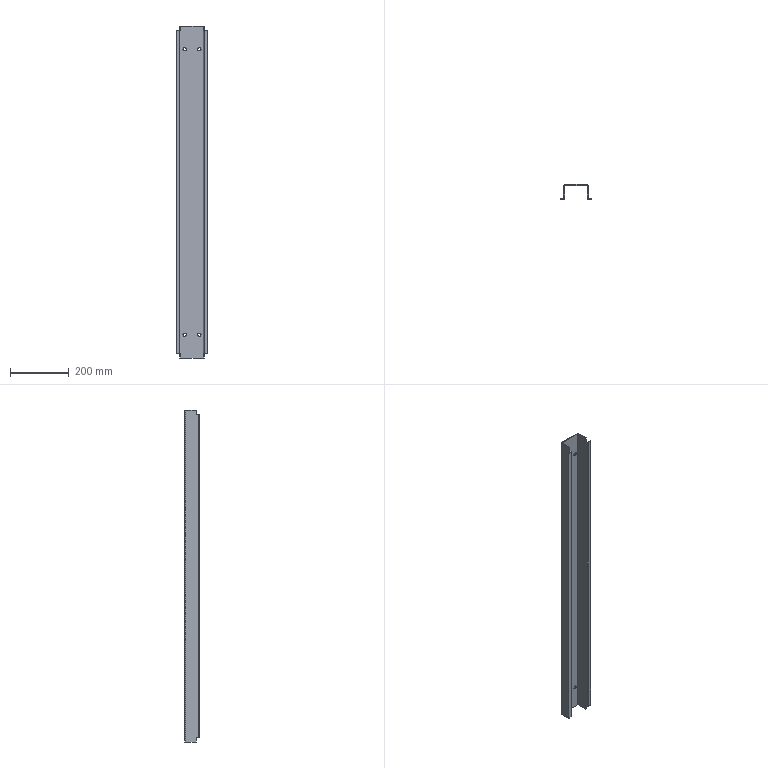Part | SolidWorks | features ICE 3, Chamfer 1, Cut 1, FlatPattern 1, SMBaseFlange 1, SheetMetal 1 | 1 solid | 54 faces | box 106 x 50 x 1127 mm | volume 661257 mm3 | plane 38 | cylinder 16 | commonest cylinder face diameters 11.5 x8 0.4 x4 6.4 x4
STEP:
#1=CARTESIAN_POINT('',(-25.,-3.,478.75));
#2=VERTEX_POINT('',#1);
#3=CARTESIAN_POINT('',(-25.,-3.,490.25));
#4=VERTEX_POINT('',#3);
#5=CARTESIAN_POINT('',(-25.,-3.,484.5));
#6=DIRECTION('',(0.,1.,0.));
#7=DIRECTION('',(-1.,0.,0.));
#8=AXIS2_PLACEMENT_3D('',#5,#6,#7);
#9=CIRCLE('',#8,5.75);
#10=EDGE_CURVE('',#2,#4,#9,.T.);
#11=ORIENTED_EDGE('',*,*,#10,.F.);
#12=CARTESIAN_POINT('',(-25.,0.,478.75));
#13=VERTEX_POINT('',#12);
#14=CARTESIAN_POINT('',(-25.,-10.,478.75));
#15=DIRECTION('',(0.,1.,0.));
#16=VECTOR('',#15,1000.);
#17=LINE('',#14,#16);
#18=EDGE_CURVE('',#2,#13,#17,.T.);
#19=ORIENTED_EDGE('',*,*,#18,.T.);
#20=CARTESIAN_POINT('',(-25.,0.,490.25));
#21=VERTEX_POINT('',#20);
#22=CARTESIAN_POINT('',(-25.,0.,484.5));
#23=DIRECTION('',(0.,1.,0.));
#24=DIRECTION('',(0.,0.,1.));
#25=AXIS2_PLACEMENT_3D('',#22,#23,#24);
#26=CIRCLE('',#25,5.75);
#27=EDGE_CURVE('',#13,#21,#26,.T.);
#28=ORIENTED_EDGE('',*,*,#27,.T.);
#29=CARTESIAN_POINT('',(-25.,-10.,490.25));
#30=DIRECTION('',(0.,1.,0.));
#31=VECTOR('',#30,1000.);
#32=LINE('',#29,#31);
#33=EDGE_CURVE('',#4,#21,#32,.T.);
#34=ORIENTED_EDGE('',*,*,#33,.F.);
#35=EDGE_LOOP('',(#11,#19,#28,#34));
#36=FACE_OUTER_BOUND('',#35,.T.);
#37=CARTESIAN_POINT('',(-25.,-10.,484.5));
#38=DIRECTION('',(0.,1.,0.));
#39=DIRECTION('',(0.,0.,1.));
#40=AXIS2_PLACEMENT_3D('',#37,#38,#39);
#41=CYLINDRICAL_SURFACE('',#40,5.75);
#42=ADVANCED_FACE('',(#36),#41,.F.);
#43=CARTESIAN_POINT('',(25.,-3.,-490.25));
#44=VERTEX_POINT('',#43);
#45=CARTESIAN_POINT('',(25.,-3.,-478.75));
#46=VERTEX_POINT('',#45);
#47=CARTESIAN_POINT('',(25.,-3.,-484.5));
#48=DIRECTION('',(0.,1.,0.));
#49=DIRECTION('',(-1.,0.,0.));
#50=AXIS2_PLACEMENT_3D('',#47,#48,#49);
#51=CIRCLE('',#50,5.75);
#52=EDGE_CURVE('',#44,#46,#51,.T.);
#53=ORIENTED_EDGE('',*,*,#52,.F.);
#54=CARTESIAN_POINT('',(25.,0.,-490.25));
#55=VERTEX_POINT('',#54);
#56=CARTESIAN_POINT('',(25.,-10.,-490.25));
#57=DIRECTION('',(0.,1.,0.));
#58=VECTOR('',#57,1000.);
#59=LINE('',#56,#58);
#60=EDGE_CURVE('',#44,#55,#59,.T.);
#61=ORIENTED_EDGE('',*,*,#60,.T.);
#62=CARTESIAN_POINT('',(25.,0.,-478.75));
#63=VERTEX_POINT('',#62);
#64=CARTESIAN_POINT('',(25.,0.,-484.5));
#65=DIRECTION('',(0.,1.,0.));
#66=DIRECTION('',(0.,0.,1.));
#67=AXIS2_PLACEMENT_3D('',#64,#65,#66);
#68=CIRCLE('',#67,5.75);
#69=EDGE_CURVE('',#55,#63,#68,.T.);
#70=ORIENTED_EDGE('',*,*,#69,.T.);
#71=CARTESIAN_POINT('',(25.,-10.,-478.75));
#72=DIRECTION('',(0.,1.,0.));
#73=VECTOR('',#72,1000.);
#74=LINE('',#71,#73);
#75=EDGE_CURVE('',#46,#63,#74,.T.);
#76=ORIENTED_EDGE('',*,*,#75,.F.);
#77=EDGE_LOOP('',(#53,#61,#70,#76));
#78=FACE_OUTER_BOUND('',#77,.T.);
#79=CARTESIAN_POINT('',(25.,-10.,-484.5));
#80=DIRECTION('',(0.,1.,0.));
#81=DIRECTION('',(0.,0.,1.));
#82=AXIS2_PLACEMENT_3D('',#79,#80,#81);
#83=CYLINDRICAL_SURFACE('',#82,5.75);
#84=ADVANCED_FACE('',(#78),#83,.F.);
#85=CARTESIAN_POINT('',(25.,-3.,478.75));
#86=VERTEX_POINT('',#85);
#87=CARTESIAN_POINT('',(25.,-3.,490.25));
#88=VERTEX_POINT('',#87);
#89=CARTESIAN_POINT('',(25.,-3.,484.5));
#90=DIRECTION('',(0.,1.,0.));
#91=DIRECTION('',(-1.,0.,0.));
#92=AXIS2_PLACEMENT_3D('',#89,#90,#91);
#93=CIRCLE('',#92,5.75);
#94=EDGE_CURVE('',#86,#88,#93,.T.);
#95=ORIENTED_EDGE('',*,*,#94,.F.);
#96=CARTESIAN_POINT('',(25.,0.,478.75));
#97=VERTEX_POINT('',#96);
#98=CARTESIAN_POINT('',(25.,-10.,478.75));
#99=DIRECTION('',(0.,1.,0.));
#100=VECTOR('',#99,1000.);
#101=LINE('',#98,#100);
#102=EDGE_CURVE('',#86,#97,#101,.T.);
#103=ORIENTED_EDGE('',*,*,#102,.T.);
#104=CARTESIAN_POINT('',(25.,0.,490.25));
#105=VERTEX_POINT('',#104);
#106=CARTESIAN_POINT('',(25.,0.,484.5));
#107=DIRECTION('',(0.,1.,0.));
#108=DIRECTION('',(0.,0.,-1.));
#109=AXIS2_PLACEMENT_3D('',#106,#107,#108);
#110=CIRCLE('',#109,5.75);
#111=EDGE_CURVE('',#97,#105,#110,.T.);
#112=ORIENTED_EDGE('',*,*,#111,.T.);
#113=CARTESIAN_POINT('',(25.,-10.,490.25));
#114=DIRECTION('',(0.,1.,0.));
#115=VECTOR('',#114,1000.);
#116=LINE('',#113,#115);
#117=EDGE_CURVE('',#88,#105,#116,.T.);
#118=ORIENTED_EDGE('',*,*,#117,.F.);
#119=EDGE_LOOP('',(#95,#103,#112,#118));
#120=FACE_OUTER_BOUND('',#119,.T.);
#121=CARTESIAN_POINT('',(25.,-10.,484.5));
#122=DIRECTION('',(0.,1.,0.));
#123=DIRECTION('',(0.,0.,1.));
#124=AXIS2_PLACEMENT_3D('',#121,#122,#123);
#125=CYLINDRICAL_SURFACE('',#124,5.75);
#126=ADVANCED_FACE('',(#120),#125,.F.);
#127=CARTESIAN_POINT('',(-25.,-3.,-490.25));
#128=VERTEX_POINT('',#127);
#129=CARTESIAN_POINT('',(-25.,-3.,-478.75));
#130=VERTEX_POINT('',#129);
#131=CARTESIAN_POINT('',(-25.,-3.,-484.5));
#132=DIRECTION('',(0.,1.,0.));
#133=DIRECTION('',(-1.,0.,0.));
#134=AXIS2_PLACEMENT_3D('',#131,#132,#133);
#135=CIRCLE('',#134,5.75);
#136=EDGE_CURVE('',#128,#130,#135,.T.);
#137=ORIENTED_EDGE('',*,*,#136,.F.);
#138=CARTESIAN_POINT('',(-25.,0.,-490.25));
#139=VERTEX_POINT('',#138);
#140=CARTESIAN_POINT('',(-25.,-10.,-490.25));
#141=DIRECTION('',(0.,1.,0.));
#142=VECTOR('',#141,1000.);
#143=LINE('',#140,#142);
#144=EDGE_CURVE('',#128,#139,#143,.T.);
#145=ORIENTED_EDGE('',*,*,#144,.T.);
#146=CARTESIAN_POINT('',(-25.,0.,-478.75));
#147=VERTEX_POINT('',#146);
#148=CARTESIAN_POINT('',(-25.,0.,-484.5));
#149=DIRECTION('',(0.,1.,0.));
#150=DIRECTION('',(0.,0.,-1.));
#151=AXIS2_PLACEMENT_3D('',#148,#149,#150);
#152=CIRCLE('',#151,5.75);
#153=EDGE_CURVE('',#139,#147,#152,.T.);
#154=ORIENTED_EDGE('',*,*,#153,.T.);
#155=CARTESIAN_POINT('',(-25.,-10.,-478.75));
#156=DIRECTION('',(0.,1.,0.));
#157=VECTOR('',#156,1000.);
#158=LINE('',#155,#157);
#159=EDGE_CURVE('',#130,#147,#158,.T.);
#160=ORIENTED_EDGE('',*,*,#159,.F.);
#161=EDGE_LOOP('',(#137,#145,#154,#160));
#162=FACE_OUTER_BOUND('',#161,.T.);
#163=CARTESIAN_POINT('',(-25.,-10.,-484.5));
#164=DIRECTION('',(0.,1.,0.));
#165=DIRECTION('',(0.,0.,1.));
#166=AXIS2_PLACEMENT_3D('',#163,#164,#165);
#167=CYLINDRICAL_SURFACE('',#166,5.75);
#168=ADVANCED_FACE('',(#162),#167,.F.);
#169=CARTESIAN_POINT('',(-53.,-50.,548.5));
#170=VERTEX_POINT('',#169);
#171=CARTESIAN_POINT('',(-41.2,-50.,548.5));
#172=VERTEX_POINT('',#171);
#173=CARTESIAN_POINT('',(-53.,-50.,548.5));
#174=DIRECTION('',(1.,0.,0.));
#175=VECTOR('',#174,1000.);
#176=LINE('',#173,#175);
#177=EDGE_CURVE('',#170,#172,#176,.T.);
#178=ORIENTED_EDGE('',*,*,#177,.T.);
#179=CARTESIAN_POINT('',(-41.2,-47.,548.5));
#180=VERTEX_POINT('',#179);
#181=CARTESIAN_POINT('',(-41.2,-50.,548.5));
#182=DIRECTION('',(0.,1.,0.));
#183=VECTOR('',#182,1000.);
#184=LINE('',#181,#183);
#185=EDGE_CURVE('',#172,#180,#184,.T.);
#186=ORIENTED_EDGE('',*,*,#185,.T.);
#187=CARTESIAN_POINT('',(-53.,-47.,548.5));
#188=VERTEX_POINT('',#187);
#189=CARTESIAN_POINT('',(-53.,-47.,548.5));
#190=DIRECTION('',(-1.,0.,0.));
#191=VECTOR('',#190,1000.);
#192=LINE('',#189,#191);
#193=EDGE_CURVE('',#180,#188,#192,.T.);
#194=ORIENTED_EDGE('',*,*,#193,.T.);
#195=CARTESIAN_POINT('',(-53.,-40.,548.5));
#196=DIRECTION('',(0.,-1.,0.));
#197=VECTOR('',#196,1000.);
#198=LINE('',#195,#197);
#199=EDGE_CURVE('',#188,#170,#198,.T.);
#200=ORIENTED_EDGE('',*,*,#199,.T.);
#201=EDGE_LOOP('',(#178,#186,#194,#200));
#202=FACE_OUTER_BOUND('',#201,.T.);
#203=CARTESIAN_POINT('',(-53.,-40.,548.5));
#204=DIRECTION('',(0.,0.,-1.));
#205=DIRECTION('',(-1.,0.,0.));
#206=AXIS2_PLACEMENT_3D('',#203,#204,#205);
#207=PLANE('',#206);
#208=ADVANCED_FACE('',(#202),#207,.F.);
#209=CARTESIAN_POINT('',(-41.,-40.,548.5));
#210=VERTEX_POINT('',#209);
#211=CARTESIAN_POINT('',(-41.,-46.8,548.5));
#212=VERTEX_POINT('',#211);
#213=CARTESIAN_POINT('',(-41.,-47.,548.5));
#214=DIRECTION('',(0.,-1.,0.));
#215=VECTOR('',#214,1000.);
#216=LINE('',#213,#215);
#217=EDGE_CURVE('',#210,#212,#216,.T.);
#218=ORIENTED_EDGE('',*,*,#217,.T.);
#219=CARTESIAN_POINT('',(-38.,-46.8,548.5));
#220=VERTEX_POINT('',#219);
#221=CARTESIAN_POINT('',(-41.,-46.8,548.5));
#222=DIRECTION('',(1.,0.,0.));
#223=VECTOR('',#222,1000.);
#224=LINE('',#221,#223);
#225=EDGE_CURVE('',#212,#220,#224,.T.);
#226=ORIENTED_EDGE('',*,*,#225,.T.);
#227=CARTESIAN_POINT('',(-38.,-40.,548.5));
#228=VERTEX_POINT('',#227);
#229=CARTESIAN_POINT('',(-38.,-47.,548.5));
#230=DIRECTION('',(0.,-1.,0.));
#231=VECTOR('',#230,1000.);
#232=LINE('',#229,#231);
#233=EDGE_CURVE('',#228,#220,#232,.T.);
#234=ORIENTED_EDGE('',*,*,#233,.F.);
#235=CARTESIAN_POINT('',(-53.,-40.,548.5));
#236=DIRECTION('',(1.,0.,0.));
#237=VECTOR('',#236,1000.);
#238=LINE('',#235,#237);
#239=EDGE_CURVE('',#210,#228,#238,.T.);
#240=ORIENTED_EDGE('',*,*,#239,.F.);
#241=EDGE_LOOP('',(#218,#226,#234,#240));
#242=FACE_OUTER_BOUND('',#241,.T.);
#243=CARTESIAN_POINT('',(-53.,-40.,548.5));
#244=DIRECTION('',(0.,0.,-1.));
#245=DIRECTION('',(-1.,0.,0.));
#246=AXIS2_PLACEMENT_3D('',#243,#244,#245);
#247=PLANE('',#246);
#248=ADVANCED_FACE('',(#242),#247,.F.);
#249=CARTESIAN_POINT('',(-53.,-47.,-548.5));
#250=VERTEX_POINT('',#249);
#251=CARTESIAN_POINT('',(-41.2,-47.,-548.5));
#252=VERTEX_POINT('',#251);
#253=CARTESIAN_POINT('',(-53.,-47.,-548.5));
#254=DIRECTION('',(1.,0.,0.));
#255=VECTOR('',#254,1000.);
#256=LINE('',#253,#255);
#257=EDGE_CURVE('',#250,#252,#256,.T.);
#258=ORIENTED_EDGE('',*,*,#257,.T.);
#259=CARTESIAN_POINT('',(-41.2,-50.,-548.5));
#260=VERTEX_POINT('',#259);
#261=CARTESIAN_POINT('',(-41.2,-47.,-548.5));
#262=DIRECTION('',(0.,-1.,0.));
#263=VECTOR('',#262,1000.);
#264=LINE('',#261,#263);
#265=EDGE_CURVE('',#252,#260,#264,.T.);
#266=ORIENTED_EDGE('',*,*,#265,.T.);
#267=CARTESIAN_POINT('',(-53.,-50.,-548.5));
#268=VERTEX_POINT('',#267);
#269=CARTESIAN_POINT('',(-53.,-50.,-548.5));
#270=DIRECTION('',(-1.,0.,0.));
#271=VECTOR('',#270,1000.);
#272=LINE('',#269,#271);
#273=EDGE_CURVE('',#260,#268,#272,.T.);
#274=ORIENTED_EDGE('',*,*,#273,.T.);
#275=CARTESIAN_POINT('',(-53.,-40.,-548.5));
#276=DIRECTION('',(0.,-1.,0.));
#277=VECTOR('',#276,1000.);
#278=LINE('',#275,#277);
#279=EDGE_CURVE('',#250,#268,#278,.T.);
#280=ORIENTED_EDGE('',*,*,#279,.F.);
#281=EDGE_LOOP('',(#258,#266,#274,#280));
#282=FACE_OUTER_BOUND('',#281,.T.);
#283=CARTESIAN_POINT('',(-53.,-40.,-548.5));
#284=DIRECTION('',(0.,0.,1.));
#285=DIRECTION('',(1.,0.,0.));
#286=AXIS2_PLACEMENT_3D('',#283,#284,#285);
#287=PLANE('',#286);
#288=ADVANCED_FACE('',(#282),#287,.F.);
#289=CARTESIAN_POINT('',(-38.,-46.8,-548.5));
#290=VERTEX_POINT('',#289);
#291=CARTESIAN_POINT('',(-38.,-40.,-548.5));
#292=VERTEX_POINT('',#291);
#293=CARTESIAN_POINT('',(-38.,-47.,-548.5));
#294=DIRECTION('',(0.,1.,0.));
#295=VECTOR('',#294,1000.);
#296=LINE('',#293,#295);
#297=EDGE_CURVE('',#290,#292,#296,.T.);
#298=ORIENTED_EDGE('',*,*,#297,.F.);
#299=CARTESIAN_POINT('',(-41.,-46.8,-548.5));
#300=VERTEX_POINT('',#299);
#301=CARTESIAN_POINT('',(-38.,-46.8,-548.5));
#302=DIRECTION('',(-1.,0.,0.));
#303=VECTOR('',#302,1000.);
#304=LINE('',#301,#303);
#305=EDGE_CURVE('',#290,#300,#304,.T.);
#306=ORIENTED_EDGE('',*,*,#305,.T.);
#307=CARTESIAN_POINT('',(-41.,-40.,-548.5));
#308=VERTEX_POINT('',#307);
#309=CARTESIAN_POINT('',(-41.,-47.,-548.5));
#310=DIRECTION('',(0.,1.,0.));
#311=VECTOR('',#310,1000.);
#312=LINE('',#309,#311);
#313=EDGE_CURVE('',#300,#308,#312,.T.);
#314=ORIENTED_EDGE('',*,*,#313,.T.);
#315=CARTESIAN_POINT('',(-53.,-40.,-548.5));
#316=DIRECTION('',(-1.,0.,0.));
#317=VECTOR('',#316,1000.);
#318=LINE('',#315,#317);
#319=EDGE_CURVE('',#292,#308,#318,.T.);
#320=ORIENTED_EDGE('',*,*,#319,.F.);
#321=EDGE_LOOP('',(#298,#306,#314,#320));
#322=FACE_OUTER_BOUND('',#321,.T.);
#323=CARTESIAN_POINT('',(-53.,-40.,-548.5));
#324=DIRECTION('',(0.,0.,1.));
#325=DIRECTION('',(1.,0.,0.));
#326=AXIS2_PLACEMENT_3D('',#323,#324,#325);
#327=PLANE('',#326);
#328=ADVANCED_FACE('',(#322),#327,.F.);
#329=CARTESIAN_POINT('',(38.,-46.8,548.5));
#330=VERTEX_POINT('',#329);
#331=CARTESIAN_POINT('',(38.,-40.,548.5));
#332=VERTEX_POINT('',#331);
#333=CARTESIAN_POINT('',(38.,0.,548.5));
#334=DIRECTION('',(0.,1.,0.));
#335=VECTOR('',#334,1000.);
#336=LINE('',#333,#335);
#337=EDGE_CURVE('',#330,#332,#336,.T.);
#338=ORIENTED_EDGE('',*,*,#337,.F.);
#339=CARTESIAN_POINT('',(41.,-46.8,548.5));
#340=VERTEX_POINT('',#339);
#341=CARTESIAN_POINT('',(38.,-46.8,548.5));
#342=DIRECTION('',(1.,0.,0.));
#343=VECTOR('',#342,1000.);
#344=LINE('',#341,#343);
#345=EDGE_CURVE('',#330,#340,#344,.T.);
#346=ORIENTED_EDGE('',*,*,#345,.T.);
#347=CARTESIAN_POINT('',(41.,-40.,548.5));
#348=VERTEX_POINT('',#347);
#349=CARTESIAN_POINT('',(41.,0.,548.5));
#350=DIRECTION('',(0.,1.,0.));
#351=VECTOR('',#350,1000.);
#352=LINE('',#349,#351);
#353=EDGE_CURVE('',#340,#348,#352,.T.);
#354=ORIENTED_EDGE('',*,*,#353,.T.);
#355=CARTESIAN_POINT('',(-53.,-40.,548.5));
#356=DIRECTION('',(1.,0.,0.));
#357=VECTOR('',#356,1000.);
#358=LINE('',#355,#357);
#359=EDGE_CURVE('',#332,#348,#358,.T.);
#360=ORIENTED_EDGE('',*,*,#359,.F.);
#361=EDGE_LOOP('',(#338,#346,#354,#360));
#362=FACE_OUTER_BOUND('',#361,.T.);
#363=CARTESIAN_POINT('',(-53.,-40.,548.5));
#364=DIRECTION('',(0.,0.,-1.));
#365=DIRECTION('',(-1.,0.,0.));
#366=AXIS2_PLACEMENT_3D('',#363,#364,#365);
#367=PLANE('',#366);
#368=ADVANCED_FACE('',(#362),#367,.F.);
#369=CARTESIAN_POINT('',(53.,-47.,548.5));
#370=VERTEX_POINT('',#369);
#371=CARTESIAN_POINT('',(41.2,-47.,548.5));
#372=VERTEX_POINT('',#371);
#373=CARTESIAN_POINT('',(41.,-47.,548.5));
#374=DIRECTION('',(-1.,0.,0.));
#375=VECTOR('',#374,1000.);
#376=LINE('',#373,#375);
#377=EDGE_CURVE('',#370,#372,#376,.T.);
#378=ORIENTED_EDGE('',*,*,#377,.T.);
#379=CARTESIAN_POINT('',(41.2,-50.,548.5));
#380=VERTEX_POINT('',#379);
#381=CARTESIAN_POINT('',(41.2,-47.,548.5));
#382=DIRECTION('',(0.,-1.,0.));
#383=VECTOR('',#382,1000.);
#384=LINE('',#381,#383);
#385=EDGE_CURVE('',#372,#380,#384,.T.);
#386=ORIENTED_EDGE('',*,*,#385,.T.);
#387=CARTESIAN_POINT('',(53.,-50.,548.5));
#388=VERTEX_POINT('',#387);
#389=CARTESIAN_POINT('',(-53.,-50.,548.5));
#390=DIRECTION('',(1.,0.,0.));
#391=VECTOR('',#390,1000.);
#392=LINE('',#389,#391);
#393=EDGE_CURVE('',#380,#388,#392,.T.);
#394=ORIENTED_EDGE('',*,*,#393,.T.);
#395=CARTESIAN_POINT('',(53.,-40.,548.5));
#396=DIRECTION('',(0.,-1.,0.));
#397=VECTOR('',#396,1000.);
#398=LINE('',#395,#397);
#399=EDGE_CURVE('',#370,#388,#398,.T.);
#400=ORIENTED_EDGE('',*,*,#399,.F.);
#401=EDGE_LOOP('',(#378,#386,#394,#400));
#402=FACE_OUTER_BOUND('',#401,.T.);
#403=CARTESIAN_POINT('',(-53.,-40.,548.5));
#404=DIRECTION('',(0.,0.,-1.));
#405=DIRECTION('',(-1.,0.,0.));
#406=AXIS2_PLACEMENT_3D('',#403,#404,#405);
#407=PLANE('',#406);
#408=ADVANCED_FACE('',(#402),#407,.F.);
#409=CARTESIAN_POINT('',(41.,-40.,-548.5));
#410=VERTEX_POINT('',#409);
#411=CARTESIAN_POINT('',(41.,-46.8,-548.5));
#412=VERTEX_POINT('',#411);
#413=CARTESIAN_POINT('',(41.,0.,-548.5));
#414=DIRECTION('',(0.,-1.,0.));
#415=VECTOR('',#414,1000.);
#416=LINE('',#413,#415);
#417=EDGE_CURVE('',#410,#412,#416,.T.);
#418=ORIENTED_EDGE('',*,*,#417,.T.);
#419=CARTESIAN_POINT('',(38.,-46.8,-548.5));
#420=VERTEX_POINT('',#419);
#421=CARTESIAN_POINT('',(41.,-46.8,-548.5));
#422=DIRECTION('',(-1.,0.,0.));
#423=VECTOR('',#422,1000.);
#424=LINE('',#421,#423);
#425=EDGE_CURVE('',#412,#420,#424,.T.);
#426=ORIENTED_EDGE('',*,*,#425,.T.);
#427=CARTESIAN_POINT('',(38.,-40.,-548.5));
#428=VERTEX_POINT('',#427);
#429=CARTESIAN_POINT('',(38.,0.,-548.5));
#430=DIRECTION('',(0.,-1.,0.));
#431=VECTOR('',#430,1000.);
#432=LINE('',#429,#431);
#433=EDGE_CURVE('',#428,#420,#432,.T.);
#434=ORIENTED_EDGE('',*,*,#433,.F.);
#435=CARTESIAN_POINT('',(-53.,-40.,-548.5));
#436=DIRECTION('',(-1.,0.,0.));
#437=VECTOR('',#436,1000.);
#438=LINE('',#435,#437);
#439=EDGE_CURVE('',#410,#428,#438,.T.);
#440=ORIENTED_EDGE('',*,*,#439,.F.);
#441=EDGE_LOOP('',(#418,#426,#434,#440));
#442=FACE_OUTER_BOUND('',#441,.T.);
#443=CARTESIAN_POINT('',(-53.,-40.,-548.5));
#444=DIRECTION('',(0.,0.,1.));
#445=DIRECTION('',(1.,0.,0.));
#446=AXIS2_PLACEMENT_3D('',#443,#444,#445);
#447=PLANE('',#446);
#448=ADVANCED_FACE('',(#442),#447,.F.);
#449=CARTESIAN_POINT('',(53.,-50.,-548.5));
#450=VERTEX_POINT('',#449);
#451=CARTESIAN_POINT('',(41.2,-50.,-548.5));
#452=VERTEX_POINT('',#451);
#453=CARTESIAN_POINT('',(-53.,-50.,-548.5));
#454=DIRECTION('',(-1.,0.,0.));
#455=VECTOR('',#454,1000.);
#456=LINE('',#453,#455);
#457=EDGE_CURVE('',#450,#452,#456,.T.);
#458=ORIENTED_EDGE('',*,*,#457,.T.);
#459=CARTESIAN_POINT('',(41.2,-47.,-548.5));
#460=VERTEX_POINT('',#459);
#461=CARTESIAN_POINT('',(41.2,-50.,-548.5));
#462=DIRECTION('',(0.,1.,0.));
#463=VECTOR('',#462,1000.);
#464=LINE('',#461,#463);
#465=EDGE_CURVE('',#452,#460,#464,.T.);
#466=ORIENTED_EDGE('',*,*,#465,.T.);
#467=CARTESIAN_POINT('',(53.,-47.,-548.5));
#468=VERTEX_POINT('',#467);
#469=CARTESIAN_POINT('',(41.,-47.,-548.5));
#470=DIRECTION('',(1.,0.,0.));
#471=VECTOR('',#470,1000.);
#472=LINE('',#469,#471);
#473=EDGE_CURVE('',#460,#468,#472,.T.);
#474=ORIENTED_EDGE('',*,*,#473,.T.);
#475=CARTESIAN_POINT('',(53.,-40.,-548.5));
#476=DIRECTION('',(0.,-1.,0.));
#477=VECTOR('',#476,1000.);
#478=LINE('',#475,#477);
#479=EDGE_CURVE('',#468,#450,#478,.T.);
#480=ORIENTED_EDGE('',*,*,#479,.T.);
#481=EDGE_LOOP('',(#458,#466,#474,#480));
#482=FACE_OUTER_BOUND('',#481,.T.);
#483=CARTESIAN_POINT('',(-53.,-40.,-548.5));
#484=DIRECTION('',(0.,0.,1.));
#485=DIRECTION('',(1.,0.,0.));
#486=AXIS2_PLACEMENT_3D('',#483,#484,#485);
#487=PLANE('',#486);
#488=ADVANCED_FACE('',(#482),#487,.F.);
#489=CARTESIAN_POINT('',(-41.,-40.,563.5));
#490=VERTEX_POINT('',#489);
#491=CARTESIAN_POINT('',(-41.,-3.2,563.5));
#492=VERTEX_POINT('',#491);
#493=CARTESIAN_POINT('',(-41.,-47.,563.5));
#494=DIRECTION('',(0.,1.,0.));
#495=VECTOR('',#494,1000.);
#496=LINE('',#493,#495);
#497=EDGE_CURVE('',#490,#492,#496,.T.);
#498=ORIENTED_EDGE('',*,*,#497,.F.);
#499=CARTESIAN_POINT('',(-38.,-40.,563.5));
#500=VERTEX_POINT('',#499);
#501=CARTESIAN_POINT('',(-53.,-40.,563.5));
#502=DIRECTION('',(-1.,0.,0.));
#503=VECTOR('',#502,1000.);
#504=LINE('',#501,#503);
#505=EDGE_CURVE('',#500,#490,#504,.T.);
#506=ORIENTED_EDGE('',*,*,#505,.F.);
#507=CARTESIAN_POINT('',(-38.,-3.2,563.5));
#508=VERTEX_POINT('',#507);
#509=CARTESIAN_POINT('',(-38.,-47.,563.5));
#510=DIRECTION('',(0.,1.,0.));
#511=VECTOR('',#510,1000.);
#512=LINE('',#509,#511);
#513=EDGE_CURVE('',#500,#508,#512,.T.);
#514=ORIENTED_EDGE('',*,*,#513,.T.);
#515=CARTESIAN_POINT('',(-38.,-3.2,563.5));
#516=DIRECTION('',(-1.,0.,0.));
#517=VECTOR('',#516,1000.);
#518=LINE('',#515,#517);
#519=EDGE_CURVE('',#508,#492,#518,.T.);
#520=ORIENTED_EDGE('',*,*,#519,.T.);
#521=EDGE_LOOP('',(#498,#506,#514,#520));
#522=FACE_OUTER_BOUND('',#521,.T.);
#523=CARTESIAN_POINT('',(-41.2,-50.,563.5));
#524=DIRECTION('',(0.,0.,1.));
#525=DIRECTION('',(1.,0.,0.));
#526=AXIS2_PLACEMENT_3D('',#523,#524,#525);
#527=PLANE('',#526);
#528=ADVANCED_FACE('',(#522),#527,.T.);
#529=CARTESIAN_POINT('',(38.,-3.2,563.5));
#530=VERTEX_POINT('',#529);
#531=CARTESIAN_POINT('',(38.,-40.,563.5));
#532=VERTEX_POINT('',#531);
#533=CARTESIAN_POINT('',(38.,0.,563.5));
#534=DIRECTION('',(0.,-1.,0.));
#535=VECTOR('',#534,1000.);
#536=LINE('',#533,#535);
#537=EDGE_CURVE('',#530,#532,#536,.T.);
#538=ORIENTED_EDGE('',*,*,#537,.T.);
#539=CARTESIAN_POINT('',(41.,-40.,563.5));
#540=VERTEX_POINT('',#539);
#541=CARTESIAN_POINT('',(-53.,-40.,563.5));
#542=DIRECTION('',(-1.,0.,0.));
#543=VECTOR('',#542,1000.);
#544=LINE('',#541,#543);
#545=EDGE_CURVE('',#540,#532,#544,.T.);
#546=ORIENTED_EDGE('',*,*,#545,.F.);
#547=CARTESIAN_POINT('',(41.,-3.2,563.5));
#548=VERTEX_POINT('',#547);
#549=CARTESIAN_POINT('',(41.,0.,563.5));
#550=DIRECTION('',(0.,-1.,0.));
#551=VECTOR('',#550,1000.);
#552=LINE('',#549,#551);
#553=EDGE_CURVE('',#548,#540,#552,.T.);
#554=ORIENTED_EDGE('',*,*,#553,.F.);
#555=CARTESIAN_POINT('',(41.,-3.2,563.5));
#556=DIRECTION('',(-1.,0.,0.));
#557=VECTOR('',#556,1000.);
#558=LINE('',#555,#557);
#559=EDGE_CURVE('',#548,#530,#558,.T.);
#560=ORIENTED_EDGE('',*,*,#559,.T.);
#561=EDGE_LOOP('',(#538,#546,#554,#560));
#562=FACE_OUTER_BOUND('',#561,.T.);
#563=CARTESIAN_POINT('',(37.8,-3.,563.5));
#564=DIRECTION('',(0.,0.,1.));
#565=DIRECTION('',(1.,0.,0.));
#566=AXIS2_PLACEMENT_3D('',#563,#564,#565);
#567=PLANE('',#566);
#568=ADVANCED_FACE('',(#562),#567,.T.);
#569=CARTESIAN_POINT('',(-37.8,0.,563.5));
#570=VERTEX_POINT('',#569);
#571=CARTESIAN_POINT('',(-37.8,-3.,563.5));
#572=VERTEX_POINT('',#571);
#573=CARTESIAN_POINT('',(-37.8,0.,563.5));
#574=DIRECTION('',(0.,-1.,0.));
#575=VECTOR('',#574,1000.);
#576=LINE('',#573,#575);
#577=EDGE_CURVE('',#570,#572,#576,.T.);
#578=ORIENTED_EDGE('',*,*,#577,.F.);
#579=CARTESIAN_POINT('',(-37.8,-3.2,563.5));
#580=DIRECTION('',(0.,0.,-1.));
#581=DIRECTION('',(1.,0.,0.));
#582=AXIS2_PLACEMENT_3D('',#579,#580,#581);
#583=CIRCLE('',#582,3.2);
#584=EDGE_CURVE('',#492,#570,#583,.T.);
#585=ORIENTED_EDGE('',*,*,#584,.F.);
#586=ORIENTED_EDGE('',*,*,#519,.F.);
#587=CARTESIAN_POINT('',(-37.8,-3.2,563.5));
#588=DIRECTION('',(0.,0.,-1.));
#589=DIRECTION('',(1.,0.,0.));
#590=AXIS2_PLACEMENT_3D('',#587,#588,#589);
#591=CIRCLE('',#590,0.2);
#592=EDGE_CURVE('',#508,#572,#591,.T.);
#593=ORIENTED_EDGE('',*,*,#592,.T.);
#594=EDGE_LOOP('',(#578,#585,#586,#593));
#595=FACE_OUTER_BOUND('',#594,.T.);
#596=CARTESIAN_POINT('',(-37.8,0.,563.5));
#597=DIRECTION('',(0.,0.,1.));
#598=DIRECTION('',(1.,0.,0.));
#599=AXIS2_PLACEMENT_3D('',#596,#597,#598);
#600=PLANE('',#599);
#601=ADVANCED_FACE('',(#595),#600,.T.);
#602=CARTESIAN_POINT('',(37.8,0.,563.5));
#603=VERTEX_POINT('',#602);
#604=CARTESIAN_POINT('',(-41.,0.,563.5));
#605=DIRECTION('',(1.,0.,0.));
#606=VECTOR('',#605,1000.);
#607=LINE('',#604,#606);
#608=EDGE_CURVE('',#570,#603,#607,.T.);
#609=ORIENTED_EDGE('',*,*,#608,.F.);
#610=ORIENTED_EDGE('',*,*,#577,.T.);
#611=CARTESIAN_POINT('',(37.8,-3.,563.5));
#612=VERTEX_POINT('',#611);
#613=CARTESIAN_POINT('',(-41.,-3.,563.5));
#614=DIRECTION('',(1.,0.,0.));
#615=VECTOR('',#614,1000.);
#616=LINE('',#613,#615);
#617=EDGE_CURVE('',#572,#612,#616,.T.);
#618=ORIENTED_EDGE('',*,*,#617,.T.);
#619=CARTESIAN_POINT('',(37.8,-3.,563.5));
#620=DIRECTION('',(0.,1.,0.));
#621=VECTOR('',#620,1000.);
#622=LINE('',#619,#621);
#623=EDGE_CURVE('',#612,#603,#622,.T.);
#624=ORIENTED_EDGE('',*,*,#623,.T.);
#625=EDGE_LOOP('',(#609,#610,#618,#624));
#626=FACE_OUTER_BOUND('',#625,.T.);
#627=CARTESIAN_POINT('',(-38.,-3.2,563.5));
#628=DIRECTION('',(0.,0.,1.));
#629=DIRECTION('',(1.,0.,0.));
#630=AXIS2_PLACEMENT_3D('',#627,#628,#629);
#631=PLANE('',#630);
#632=ADVANCED_FACE('',(#626),#631,.T.);
#633=CARTESIAN_POINT('',(-41.,-3.2,-563.5));
#634=VERTEX_POINT('',#633);
#635=CARTESIAN_POINT('',(-38.,-3.2,-563.5));
#636=VERTEX_POINT('',#635);
#637=CARTESIAN_POINT('',(-41.,-3.2,-563.5));
#638=DIRECTION('',(1.,0.,0.));
#639=VECTOR('',#638,1000.);
#640=LINE('',#637,#639);
#641=EDGE_CURVE('',#634,#636,#640,.T.);
#642=ORIENTED_EDGE('',*,*,#641,.F.);
#643=CARTESIAN_POINT('',(-37.8,0.,-563.5));
#644=VERTEX_POINT('',#643);
#645=CARTESIAN_POINT('',(-37.8,-3.2,-563.5));
#646=DIRECTION('',(0.,0.,-1.));
#647=DIRECTION('',(1.,0.,0.));
#648=AXIS2_PLACEMENT_3D('',#645,#646,#647);
#649=CIRCLE('',#648,3.2);
#650=EDGE_CURVE('',#634,#644,#649,.T.);
#651=ORIENTED_EDGE('',*,*,#650,.T.);
#652=CARTESIAN_POINT('',(-37.8,-3.,-563.5));
#653=VERTEX_POINT('',#652);
#654=CARTESIAN_POINT('',(-37.8,-3.,-563.5));
#655=DIRECTION('',(0.,1.,0.));
#656=VECTOR('',#655,1000.);
#657=LINE('',#654,#656);
#658=EDGE_CURVE('',#653,#644,#657,.T.);
#659=ORIENTED_EDGE('',*,*,#658,.F.);
#660=CARTESIAN_POINT('',(-37.8,-3.2,-563.5));
#661=DIRECTION('',(0.,0.,-1.));
#662=DIRECTION('',(1.,0.,0.));
#663=AXIS2_PLACEMENT_3D('',#660,#661,#662);
#664=CIRCLE('',#663,0.2);
#665=EDGE_CURVE('',#636,#653,#664,.T.);
#666=ORIENTED_EDGE('',*,*,#665,.F.);
#667=EDGE_LOOP('',(#642,#651,#659,#666));
#668=FACE_OUTER_BOUND('',#667,.T.);
#669=CARTESIAN_POINT('',(-41.,-3.2,-563.5));
#670=DIRECTION('',(0.,0.,-1.));
#671=DIRECTION('',(-1.,0.,0.));
#672=AXIS2_PLACEMENT_3D('',#669,#670,#671);
#673=PLANE('',#672);
#674=ADVANCED_FACE('',(#668),#673,.T.);
#675=CARTESIAN_POINT('',(-41.,-40.,-563.5));
#676=VERTEX_POINT('',#675);
#677=CARTESIAN_POINT('',(-38.,-40.,-563.5));
#678=VERTEX_POINT('',#677);
#679=CARTESIAN_POINT('',(-53.,-40.,-563.5));
#680=DIRECTION('',(1.,0.,0.));
#681=VECTOR('',#680,1000.);
#682=LINE('',#679,#681);
#683=EDGE_CURVE('',#676,#678,#682,.T.);
#684=ORIENTED_EDGE('',*,*,#683,.F.);
#685=CARTESIAN_POINT('',(-41.,-47.,-563.5));
#686=DIRECTION('',(0.,1.,0.));
#687=VECTOR('',#686,1000.);
#688=LINE('',#685,#687);
#689=EDGE_CURVE('',#676,#634,#688,.T.);
#690=ORIENTED_EDGE('',*,*,#689,.T.);
#691=ORIENTED_EDGE('',*,*,#641,.T.);
#692=CARTESIAN_POINT('',(-38.,-47.,-563.5));
#693=DIRECTION('',(0.,1.,0.));
#694=VECTOR('',#693,1000.);
#695=LINE('',#692,#694);
#696=EDGE_CURVE('',#678,#636,#695,.T.);
#697=ORIENTED_EDGE('',*,*,#696,.F.);
#698=EDGE_LOOP('',(#684,#690,#691,#697));
#699=FACE_OUTER_BOUND('',#698,.T.);
#700=CARTESIAN_POINT('',(-37.8,-3.,-563.5));
#701=DIRECTION('',(0.,0.,-1.));
#702=DIRECTION('',(-1.,0.,0.));
#703=AXIS2_PLACEMENT_3D('',#700,#701,#702);
#704=PLANE('',#703);
#705=ADVANCED_FACE('',(#699),#704,.T.);
#706=ORIENTED_EDGE('',*,*,#559,.F.);
#707=CARTESIAN_POINT('',(37.8,-3.2,563.5));
#708=DIRECTION('',(0.,0.,-1.));
#709=DIRECTION('',(1.,0.,0.));
#710=AXIS2_PLACEMENT_3D('',#707,#708,#709);
#711=CIRCLE('',#710,3.2);
#712=EDGE_CURVE('',#603,#548,#711,.T.);
#713=ORIENTED_EDGE('',*,*,#712,.F.);
#714=ORIENTED_EDGE('',*,*,#623,.F.);
#715=CARTESIAN_POINT('',(37.8,-3.2,563.5));
#716=DIRECTION('',(0.,0.,-1.));
#717=DIRECTION('',(1.,0.,0.));
#718=AXIS2_PLACEMENT_3D('',#715,#716,#717);
#719=CIRCLE('',#718,0.2);
#720=EDGE_CURVE('',#612,#530,#719,.T.);
#721=ORIENTED_EDGE('',*,*,#720,.T.);
#722=EDGE_LOOP('',(#706,#713,#714,#721));
#723=FACE_OUTER_BOUND('',#722,.T.);
#724=CARTESIAN_POINT('',(41.,-3.2,563.5));
#725=DIRECTION('',(0.,0.,1.));
#726=DIRECTION('',(1.,0.,0.));
#727=AXIS2_PLACEMENT_3D('',#724,#725,#726);
#728=PLANE('',#727);
#729=ADVANCED_FACE('',(#723),#728,.T.);
#730=CARTESIAN_POINT('',(37.8,0.,-563.5));
#731=VERTEX_POINT('',#730);
#732=CARTESIAN_POINT('',(37.8,-3.,-563.5));
#733=VERTEX_POINT('',#732);
#734=CARTESIAN_POINT('',(37.8,0.,-563.5));
#735=DIRECTION('',(0.,-1.,0.));
#736=VECTOR('',#735,1000.);
#737=LINE('',#734,#736);
#738=EDGE_CURVE('',#731,#733,#737,.T.);
#739=ORIENTED_EDGE('',*,*,#738,.F.);
#740=CARTESIAN_POINT('',(41.,-3.2,-563.5));
#741=VERTEX_POINT('',#740);
#742=CARTESIAN_POINT('',(37.8,-3.2,-563.5));
#743=DIRECTION('',(0.,0.,-1.));
#744=DIRECTION('',(1.,0.,0.));
#745=AXIS2_PLACEMENT_3D('',#742,#743,#744);
#746=CIRCLE('',#745,3.2);
#747=EDGE_CURVE('',#731,#741,#746,.T.);
#748=ORIENTED_EDGE('',*,*,#747,.T.);
#749=CARTESIAN_POINT('',(38.,-3.2,-563.5));
#750=VERTEX_POINT('',#749);
#751=CARTESIAN_POINT('',(38.,-3.2,-563.5));
#752=DIRECTION('',(1.,0.,0.));
#753=VECTOR('',#752,1000.);
#754=LINE('',#751,#753);
#755=EDGE_CURVE('',#750,#741,#754,.T.);
#756=ORIENTED_EDGE('',*,*,#755,.F.);
#757=CARTESIAN_POINT('',(37.8,-3.2,-563.5));
#758=DIRECTION('',(0.,0.,-1.));
#759=DIRECTION('',(1.,0.,0.));
#760=AXIS2_PLACEMENT_3D('',#757,#758,#759);
#761=CIRCLE('',#760,0.2);
#762=EDGE_CURVE('',#733,#750,#761,.T.);
#763=ORIENTED_EDGE('',*,*,#762,.F.);
#764=EDGE_LOOP('',(#739,#748,#756,#763));
#765=FACE_OUTER_BOUND('',#764,.T.);
#766=CARTESIAN_POINT('',(37.8,0.,-563.5));
#767=DIRECTION('',(0.,0.,-1.));
#768=DIRECTION('',(-1.,0.,0.));
#769=AXIS2_PLACEMENT_3D('',#766,#767,#768);
#770=PLANE('',#769);
#771=ADVANCED_FACE('',(#765),#770,.T.);
#772=CARTESIAN_POINT('',(-41.,0.,-563.5));
#773=DIRECTION('',(1.,0.,0.));
#774=VECTOR('',#773,1000.);
#775=LINE('',#772,#774);
#776=EDGE_CURVE('',#644,#731,#775,.T.);
#777=ORIENTED_EDGE('',*,*,#776,.T.);
#778=ORIENTED_EDGE('',*,*,#738,.T.);
#779=CARTESIAN_POINT('',(-41.,-3.,-563.5));
#780=DIRECTION('',(1.,0.,0.));
#781=VECTOR('',#780,1000.);
#782=LINE('',#779,#781);
#783=EDGE_CURVE('',#653,#733,#782,.T.);
#784=ORIENTED_EDGE('',*,*,#783,.F.);
#785=ORIENTED_EDGE('',*,*,#658,.T.);
#786=EDGE_LOOP('',(#777,#778,#784,#785));
#787=FACE_OUTER_BOUND('',#786,.T.);
#788=CARTESIAN_POINT('',(38.,-3.2,-563.5));
#789=DIRECTION('',(0.,0.,-1.));
#790=DIRECTION('',(-1.,0.,0.));
#791=AXIS2_PLACEMENT_3D('',#788,#789,#790);
#792=PLANE('',#791);
#793=ADVANCED_FACE('',(#787),#792,.T.);
#794=CARTESIAN_POINT('',(38.,-40.,-563.5));
#795=VERTEX_POINT('',#794);
#796=CARTESIAN_POINT('',(41.,-40.,-563.5));
#797=VERTEX_POINT('',#796);
#798=CARTESIAN_POINT('',(-53.,-40.,-563.5));
#799=DIRECTION('',(1.,0.,0.));
#800=VECTOR('',#799,1000.);
#801=LINE('',#798,#800);
#802=EDGE_CURVE('',#795,#797,#801,.T.);
#803=ORIENTED_EDGE('',*,*,#802,.F.);
#804=CARTESIAN_POINT('',(38.,0.,-563.5));
#805=DIRECTION('',(0.,-1.,0.));
#806=VECTOR('',#805,1000.);
#807=LINE('',#804,#806);
#808=EDGE_CURVE('',#750,#795,#807,.T.);
#809=ORIENTED_EDGE('',*,*,#808,.F.);
#810=ORIENTED_EDGE('',*,*,#755,.T.);
#811=CARTESIAN_POINT('',(41.,0.,-563.5));
#812=DIRECTION('',(0.,-1.,0.));
#813=VECTOR('',#812,1000.);
#814=LINE('',#811,#813);
#815=EDGE_CURVE('',#741,#797,#814,.T.);
#816=ORIENTED_EDGE('',*,*,#815,.T.);
#817=EDGE_LOOP('',(#803,#809,#810,#816));
#818=FACE_OUTER_BOUND('',#817,.T.);
#819=CARTESIAN_POINT('',(41.2,-50.,-563.5));
#820=DIRECTION('',(0.,0.,-1.));
#821=DIRECTION('',(-1.,0.,0.));
#822=AXIS2_PLACEMENT_3D('',#819,#820,#821);
#823=PLANE('',#822);
#824=ADVANCED_FACE('',(#818),#823,.T.);
#825=CARTESIAN_POINT('',(53.,-50.,563.5));
#826=DIRECTION('',(0.,0.,-1.));
#827=VECTOR('',#826,1000.);
#828=LINE('',#825,#827);
#829=EDGE_CURVE('',#388,#450,#828,.T.);
#830=ORIENTED_EDGE('',*,*,#829,.F.);
#831=ORIENTED_EDGE('',*,*,#393,.F.);
#832=CARTESIAN_POINT('',(41.2,-50.,563.5));
#833=DIRECTION('',(0.,0.,-1.));
#834=VECTOR('',#833,1000.);
#835=LINE('',#832,#834);
#836=EDGE_CURVE('',#380,#452,#835,.T.);
#837=ORIENTED_EDGE('',*,*,#836,.T.);
#838=ORIENTED_EDGE('',*,*,#457,.F.);
#839=EDGE_LOOP('',(#830,#831,#837,#838));
#840=FACE_OUTER_BOUND('',#839,.T.);
#841=CARTESIAN_POINT('',(41.,-50.,563.5));
#842=DIRECTION('',(0.,1.,0.));
#843=DIRECTION('',(-1.,0.,0.));
#844=AXIS2_PLACEMENT_3D('',#841,#842,#843);
#845=PLANE('',#844);
#846=ADVANCED_FACE('',(#840),#845,.F.);
#847=ORIENTED_EDGE('',*,*,#399,.T.);
#848=ORIENTED_EDGE('',*,*,#829,.T.);
#849=ORIENTED_EDGE('',*,*,#479,.F.);
#850=CARTESIAN_POINT('',(53.,-47.,563.5));
#851=DIRECTION('',(0.,0.,-1.));
#852=VECTOR('',#851,1000.);
#853=LINE('',#850,#852);
#854=EDGE_CURVE('',#370,#468,#853,.T.);
#855=ORIENTED_EDGE('',*,*,#854,.F.);
#856=EDGE_LOOP('',(#847,#848,#849,#855));
#857=FACE_OUTER_BOUND('',#856,.T.);
#858=CARTESIAN_POINT('',(53.,-47.,563.5));
#859=DIRECTION('',(1.,0.,0.));
#860=DIRECTION('',(0.,0.,-1.));
#861=AXIS2_PLACEMENT_3D('',#858,#859,#860);
#862=PLANE('',#861);
#863=ADVANCED_FACE('',(#857),#862,.T.);
#864=ORIENTED_EDGE('',*,*,#377,.F.);
#865=ORIENTED_EDGE('',*,*,#854,.T.);
#866=ORIENTED_EDGE('',*,*,#473,.F.);
#867=CARTESIAN_POINT('',(41.2,-47.,563.5));
#868=DIRECTION('',(0.,0.,-1.));
#869=VECTOR('',#868,1000.);
#870=LINE('',#867,#869);
#871=EDGE_CURVE('',#372,#460,#870,.T.);
#872=ORIENTED_EDGE('',*,*,#871,.F.);
#873=EDGE_LOOP('',(#864,#865,#866,#872));
#874=FACE_OUTER_BOUND('',#873,.T.);
#875=CARTESIAN_POINT('',(41.,-47.,563.5));
#876=DIRECTION('',(0.,1.,0.));
#877=DIRECTION('',(-1.,0.,0.));
#878=AXIS2_PLACEMENT_3D('',#875,#876,#877);
#879=PLANE('',#878);
#880=ADVANCED_FACE('',(#874),#879,.T.);
#881=CARTESIAN_POINT('',(41.2,-46.8,548.5));
#882=DIRECTION('',(0.,0.,-1.));
#883=DIRECTION('',(-1.,0.,0.));
#884=AXIS2_PLACEMENT_3D('',#881,#882,#883);
#885=CIRCLE('',#884,0.2);
#886=EDGE_CURVE('',#372,#340,#885,.T.);
#887=ORIENTED_EDGE('',*,*,#886,.F.);
#888=ORIENTED_EDGE('',*,*,#871,.T.);
#889=CARTESIAN_POINT('',(41.2,-46.8,-548.5));
#890=DIRECTION('',(0.,0.,1.));
#891=DIRECTION('',(1.,0.,0.));
#892=AXIS2_PLACEMENT_3D('',#889,#890,#891);
#893=CIRCLE('',#892,0.2);
#894=EDGE_CURVE('',#412,#460,#893,.T.);
#895=ORIENTED_EDGE('',*,*,#894,.F.);
#896=CARTESIAN_POINT('',(41.,-46.8,563.5));
#897=DIRECTION('',(0.,0.,-1.));
#898=VECTOR('',#897,1000.);
#899=LINE('',#896,#898);
#900=EDGE_CURVE('',#340,#412,#899,.T.);
#901=ORIENTED_EDGE('',*,*,#900,.F.);
#902=EDGE_LOOP('',(#887,#888,#895,#901));
#903=FACE_OUTER_BOUND('',#902,.T.);
#904=CARTESIAN_POINT('',(41.2,-46.8,563.5));
#905=DIRECTION('',(0.,0.,-1.));
#906=DIRECTION('',(-1.,0.,0.));
#907=AXIS2_PLACEMENT_3D('',#904,#905,#906);
#908=CYLINDRICAL_SURFACE('',#907,0.2);
#909=ADVANCED_FACE('',(#903),#908,.F.);
#910=ORIENTED_EDGE('',*,*,#353,.F.);
#911=ORIENTED_EDGE('',*,*,#900,.T.);
#912=ORIENTED_EDGE('',*,*,#417,.F.);
#913=CARTESIAN_POINT('',(41.,-40.,563.5));
#914=DIRECTION('',(0.,0.,1.));
#915=VECTOR('',#914,1000.);
#916=LINE('',#913,#915);
#917=EDGE_CURVE('',#797,#410,#916,.T.);
#918=ORIENTED_EDGE('',*,*,#917,.F.);
#919=ORIENTED_EDGE('',*,*,#815,.F.);
#920=CARTESIAN_POINT('',(41.,-3.2,563.5));
#921=DIRECTION('',(0.,0.,-1.));
#922=VECTOR('',#921,1000.);
#923=LINE('',#920,#922);
#924=EDGE_CURVE('',#548,#741,#923,.T.);
#925=ORIENTED_EDGE('',*,*,#924,.F.);
#926=ORIENTED_EDGE('',*,*,#553,.T.);
#927=CARTESIAN_POINT('',(41.,-40.,563.5));
#928=DIRECTION('',(0.,0.,-1.));
#929=VECTOR('',#928,1000.);
#930=LINE('',#927,#929);
#931=EDGE_CURVE('',#540,#348,#930,.T.);
#932=ORIENTED_EDGE('',*,*,#931,.T.);
#933=EDGE_LOOP('',(#910,#911,#912,#918,#919,#925,#926,#932));
#934=FACE_OUTER_BOUND('',#933,.T.);
#935=CARTESIAN_POINT('',(41.,0.,563.5));
#936=DIRECTION('',(1.,0.,0.));
#937=DIRECTION('',(0.,1.,0.));
#938=AXIS2_PLACEMENT_3D('',#935,#936,#937);
#939=PLANE('',#938);
#940=ADVANCED_FACE('',(#934),#939,.T.);
#941=ORIENTED_EDGE('',*,*,#747,.F.);
#942=CARTESIAN_POINT('',(37.8,0.,563.5));
#943=DIRECTION('',(0.,0.,-1.));
#944=VECTOR('',#943,1000.);
#945=LINE('',#942,#944);
#946=EDGE_CURVE('',#603,#731,#945,.T.);
#947=ORIENTED_EDGE('',*,*,#946,.F.);
#948=ORIENTED_EDGE('',*,*,#712,.T.);
#949=ORIENTED_EDGE('',*,*,#924,.T.);
#950=EDGE_LOOP('',(#941,#947,#948,#949));
#951=FACE_OUTER_BOUND('',#950,.T.);
#952=CARTESIAN_POINT('',(37.8,-3.2,563.5));
#953=DIRECTION('',(0.,0.,-1.));
#954=DIRECTION('',(-1.,0.,0.));
#955=AXIS2_PLACEMENT_3D('',#952,#953,#954);
#956=CYLINDRICAL_SURFACE('',#955,3.2);
#957=ADVANCED_FACE('',(#951),#956,.T.);
#958=CARTESIAN_POINT('',(-25.,0.,484.5));
#959=DIRECTION('',(0.,1.,0.));
#960=DIRECTION('',(0.,0.,1.));
#961=AXIS2_PLACEMENT_3D('',#958,#959,#960);
#962=CIRCLE('',#961,5.75);
#963=EDGE_CURVE('',#21,#13,#962,.T.);
#964=ORIENTED_EDGE('',*,*,#963,.F.);
#965=ORIENTED_EDGE('',*,*,#27,.F.);
#966=EDGE_LOOP('',(#964,#965));
#967=FACE_BOUND('',#966,.T.);
#968=CARTESIAN_POINT('',(25.,0.,-484.5));
#969=DIRECTION('',(0.,1.,0.));
#970=DIRECTION('',(0.,0.,1.));
#971=AXIS2_PLACEMENT_3D('',#968,#969,#970);
#972=CIRCLE('',#971,5.75);
#973=EDGE_CURVE('',#63,#55,#972,.T.);
#974=ORIENTED_EDGE('',*,*,#973,.F.);
#975=ORIENTED_EDGE('',*,*,#69,.F.);
#976=EDGE_LOOP('',(#974,#975));
#977=FACE_BOUND('',#976,.T.);
#978=CARTESIAN_POINT('',(25.,0.,484.5));
#979=DIRECTION('',(0.,1.,0.));
#980=DIRECTION('',(0.,0.,-1.));
#981=AXIS2_PLACEMENT_3D('',#978,#979,#980);
#982=CIRCLE('',#981,5.75);
#983=EDGE_CURVE('',#105,#97,#982,.T.);
#984=ORIENTED_EDGE('',*,*,#983,.F.);
#985=ORIENTED_EDGE('',*,*,#111,.F.);
#986=EDGE_LOOP('',(#984,#985));
#987=FACE_BOUND('',#986,.T.);
#988=CARTESIAN_POINT('',(-25.,0.,-484.5));
#989=DIRECTION('',(0.,1.,0.));
#990=DIRECTION('',(0.,0.,-1.));
#991=AXIS2_PLACEMENT_3D('',#988,#989,#990);
#992=CIRCLE('',#991,5.75);
#993=EDGE_CURVE('',#147,#139,#992,.T.);
#994=ORIENTED_EDGE('',*,*,#993,.F.);
#995=ORIENTED_EDGE('',*,*,#153,.F.);
#996=EDGE_LOOP('',(#994,#995));
#997=FACE_BOUND('',#996,.T.);
#998=ORIENTED_EDGE('',*,*,#776,.F.);
#999=CARTESIAN_POINT('',(-37.8,0.,563.5));
#1000=DIRECTION('',(0.,0.,-1.));
#1001=VECTOR('',#1000,1000.);
#1002=LINE('',#999,#1001);
#1003=EDGE_CURVE('',#570,#644,#1002,.T.);
#1004=ORIENTED_EDGE('',*,*,#1003,.F.);
#1005=ORIENTED_EDGE('',*,*,#608,.T.);
#1006=ORIENTED_EDGE('',*,*,#946,.T.);
#1007=EDGE_LOOP('',(#998,#1004,#1005,#1006));
#1008=FACE_OUTER_BOUND('',#1007,.T.);
#1009=CARTESIAN_POINT('',(-41.,0.,563.5));
#1010=DIRECTION('',(0.,1.,0.));
#1011=DIRECTION('',(-1.,0.,0.));
#1012=AXIS2_PLACEMENT_3D('',#1009,#1010,#1011);
#1013=PLANE('',#1012);
#1014=ADVANCED_FACE('',(#967,#977,#987,#997,#1008),#1013,.T.);
#1015=ORIENTED_EDGE('',*,*,#650,.F.);
#1016=CARTESIAN_POINT('',(-41.,-3.2,563.5));
#1017=DIRECTION('',(0.,0.,-1.));
#1018=VECTOR('',#1017,1000.);
#1019=LINE('',#1016,#1018);
#1020=EDGE_CURVE('',#492,#634,#1019,.T.);
#1021=ORIENTED_EDGE('',*,*,#1020,.F.);
#1022=ORIENTED_EDGE('',*,*,#584,.T.);
#1023=ORIENTED_EDGE('',*,*,#1003,.T.);
#1024=EDGE_LOOP('',(#1015,#1021,#1022,#1023));
#1025=FACE_OUTER_BOUND('',#1024,.T.);
#1026=CARTESIAN_POINT('',(-37.8,-3.2,563.5));
#1027=DIRECTION('',(0.,0.,-1.));
#1028=DIRECTION('',(-1.,0.,0.));
#1029=AXIS2_PLACEMENT_3D('',#1026,#1027,#1028);
#1030=CYLINDRICAL_SURFACE('',#1029,3.2);
#1031=ADVANCED_FACE('',(#1025),#1030,.T.);
#1032=ORIENTED_EDGE('',*,*,#217,.F.);
#1033=CARTESIAN_POINT('',(-41.,-40.,563.5));
#1034=DIRECTION('',(0.,0.,1.));
#1035=VECTOR('',#1034,1000.);
#1036=LINE('',#1033,#1035);
#1037=EDGE_CURVE('',#210,#490,#1036,.T.);
#1038=ORIENTED_EDGE('',*,*,#1037,.T.);
#1039=ORIENTED_EDGE('',*,*,#497,.T.);
#1040=ORIENTED_EDGE('',*,*,#1020,.T.);
#1041=ORIENTED_EDGE('',*,*,#689,.F.);
#1042=CARTESIAN_POINT('',(-41.,-40.,563.5));
#1043=DIRECTION('',(0.,0.,-1.));
#1044=VECTOR('',#1043,1000.);
#1045=LINE('',#1042,#1044);
#1046=EDGE_CURVE('',#308,#676,#1045,.T.);
#1047=ORIENTED_EDGE('',*,*,#1046,.F.);
#1048=ORIENTED_EDGE('',*,*,#313,.F.);
#1049=CARTESIAN_POINT('',(-41.,-46.8,563.5));
#1050=DIRECTION('',(0.,0.,-1.));
#1051=VECTOR('',#1050,1000.);
#1052=LINE('',#1049,#1051);
#1053=EDGE_CURVE('',#212,#300,#1052,.T.);
#1054=ORIENTED_EDGE('',*,*,#1053,.F.);
#1055=EDGE_LOOP('',(#1032,#1038,#1039,#1040,#1041,#1047,#1048,#1054));
#1056=FACE_OUTER_BOUND('',#1055,.T.);
#1057=CARTESIAN_POINT('',(-41.,-47.,563.5));
#1058=DIRECTION('',(-1.,0.,0.));
#1059=DIRECTION('',(0.,-1.,0.));
#1060=AXIS2_PLACEMENT_3D('',#1057,#1058,#1059);
#1061=PLANE('',#1060);
#1062=ADVANCED_FACE('',(#1056),#1061,.T.);
#1063=CARTESIAN_POINT('',(-41.2,-46.8,548.5));
#1064=DIRECTION('',(0.,0.,-1.));
#1065=DIRECTION('',(-1.,0.,0.));
#1066=AXIS2_PLACEMENT_3D('',#1063,#1064,#1065);
#1067=CIRCLE('',#1066,0.2);
#1068=EDGE_CURVE('',#212,#180,#1067,.T.);
#1069=ORIENTED_EDGE('',*,*,#1068,.F.);
#1070=ORIENTED_EDGE('',*,*,#1053,.T.);
#1071=CARTESIAN_POINT('',(-41.2,-46.8,-548.5));
#1072=DIRECTION('',(0.,0.,1.));
#1073=DIRECTION('',(1.,0.,0.));
#1074=AXIS2_PLACEMENT_3D('',#1071,#1072,#1073);
#1075=CIRCLE('',#1074,0.2);
#1076=EDGE_CURVE('',#252,#300,#1075,.T.);
#1077=ORIENTED_EDGE('',*,*,#1076,.F.);
#1078=CARTESIAN_POINT('',(-41.2,-47.,563.5));
#1079=DIRECTION('',(0.,0.,-1.));
#1080=VECTOR('',#1079,1000.);
#1081=LINE('',#1078,#1080);
#1082=EDGE_CURVE('',#180,#252,#1081,.T.);
#1083=ORIENTED_EDGE('',*,*,#1082,.F.);
#1084=EDGE_LOOP('',(#1069,#1070,#1077,#1083));
#1085=FACE_OUTER_BOUND('',#1084,.T.);
#1086=CARTESIAN_POINT('',(-41.2,-46.8,563.5));
#1087=DIRECTION('',(0.,0.,-1.));
#1088=DIRECTION('',(-1.,0.,0.));
#1089=AXIS2_PLACEMENT_3D('',#1086,#1087,#1088);
#1090=CYLINDRICAL_SURFACE('',#1089,0.2);
#1091=ADVANCED_FACE('',(#1085),#1090,.F.);
#1092=ORIENTED_EDGE('',*,*,#193,.F.);
#1093=ORIENTED_EDGE('',*,*,#1082,.T.);
#1094=ORIENTED_EDGE('',*,*,#257,.F.);
#1095=CARTESIAN_POINT('',(-53.,-47.,563.5));
#1096=DIRECTION('',(0.,0.,-1.));
#1097=VECTOR('',#1096,1000.);
#1098=LINE('',#1095,#1097);
#1099=EDGE_CURVE('',#188,#250,#1098,.T.);
#1100=ORIENTED_EDGE('',*,*,#1099,.F.);
#1101=EDGE_LOOP('',(#1092,#1093,#1094,#1100));
#1102=FACE_OUTER_BOUND('',#1101,.T.);
#1103=CARTESIAN_POINT('',(-53.,-47.,563.5));
#1104=DIRECTION('',(0.,1.,0.));
#1105=DIRECTION('',(0.,0.,1.));
#1106=AXIS2_PLACEMENT_3D('',#1103,#1104,#1105);
#1107=PLANE('',#1106);
#1108=ADVANCED_FACE('',(#1102),#1107,.T.);
#1109=ORIENTED_EDGE('',*,*,#199,.F.);
#1110=ORIENTED_EDGE('',*,*,#1099,.T.);
#1111=ORIENTED_EDGE('',*,*,#279,.T.);
#1112=CARTESIAN_POINT('',(-53.,-50.,563.5));
#1113=DIRECTION('',(0.,0.,-1.));
#1114=VECTOR('',#1113,1000.);
#1115=LINE('',#1112,#1114);
#1116=EDGE_CURVE('',#170,#268,#1115,.T.);
#1117=ORIENTED_EDGE('',*,*,#1116,.F.);
#1118=EDGE_LOOP('',(#1109,#1110,#1111,#1117));
#1119=FACE_OUTER_BOUND('',#1118,.T.);
#1120=CARTESIAN_POINT('',(-53.,-50.,563.5));
#1121=DIRECTION('',(-1.,0.,0.));
#1122=DIRECTION('',(0.,0.,1.));
#1123=AXIS2_PLACEMENT_3D('',#1120,#1121,#1122);
#1124=PLANE('',#1123);
#1125=ADVANCED_FACE('',(#1119),#1124,.T.);
#1126=CARTESIAN_POINT('',(-41.2,-50.,563.5));
#1127=DIRECTION('',(0.,0.,-1.));
#1128=VECTOR('',#1127,1000.);
#1129=LINE('',#1126,#1128);
#1130=EDGE_CURVE('',#172,#260,#1129,.T.);
#1131=ORIENTED_EDGE('',*,*,#1130,.F.);
#1132=ORIENTED_EDGE('',*,*,#177,.F.);
#1133=ORIENTED_EDGE('',*,*,#1116,.T.);
#1134=ORIENTED_EDGE('',*,*,#273,.F.);
#1135=EDGE_LOOP('',(#1131,#1132,#1133,#1134));
#1136=FACE_OUTER_BOUND('',#1135,.T.);
#1137=CARTESIAN_POINT('',(-53.,-50.,563.5));
#1138=DIRECTION('',(0.,1.,0.));
#1139=DIRECTION('',(0.,0.,1.));
#1140=AXIS2_PLACEMENT_3D('',#1137,#1138,#1139);
#1141=PLANE('',#1140);
#1142=ADVANCED_FACE('',(#1136),#1141,.F.);
#1143=CARTESIAN_POINT('',(-38.,-46.8,563.5));
#1144=DIRECTION('',(0.,0.,-1.));
#1145=VECTOR('',#1144,1000.);
#1146=LINE('',#1143,#1145);
#1147=EDGE_CURVE('',#220,#290,#1146,.T.);
#1148=ORIENTED_EDGE('',*,*,#1147,.F.);
#1149=CARTESIAN_POINT('',(-41.2,-46.8,548.5));
#1150=DIRECTION('',(0.,0.,-1.));
#1151=DIRECTION('',(-1.,0.,0.));
#1152=AXIS2_PLACEMENT_3D('',#1149,#1150,#1151);
#1153=CIRCLE('',#1152,3.2);
#1154=EDGE_CURVE('',#220,#172,#1153,.T.);
#1155=ORIENTED_EDGE('',*,*,#1154,.T.);
#1156=ORIENTED_EDGE('',*,*,#1130,.T.);
#1157=CARTESIAN_POINT('',(-41.2,-46.8,-548.5));
#1158=DIRECTION('',(0.,0.,1.));
#1159=DIRECTION('',(1.,0.,0.));
#1160=AXIS2_PLACEMENT_3D('',#1157,#1158,#1159);
#1161=CIRCLE('',#1160,3.2);
#1162=EDGE_CURVE('',#260,#290,#1161,.T.);
#1163=ORIENTED_EDGE('',*,*,#1162,.T.);
#1164=EDGE_LOOP('',(#1148,#1155,#1156,#1163));
#1165=FACE_OUTER_BOUND('',#1164,.T.);
#1166=CARTESIAN_POINT('',(-41.2,-46.8,563.5));
#1167=DIRECTION('',(0.,0.,-1.));
#1168=DIRECTION('',(-1.,0.,0.));
#1169=AXIS2_PLACEMENT_3D('',#1166,#1167,#1168);
#1170=CYLINDRICAL_SURFACE('',#1169,3.2);
#1171=ADVANCED_FACE('',(#1165),#1170,.T.);
#1172=CARTESIAN_POINT('',(-38.,-40.,563.5));
#1173=DIRECTION('',(0.,0.,1.));
#1174=VECTOR('',#1173,1000.);
#1175=LINE('',#1172,#1174);
#1176=EDGE_CURVE('',#228,#500,#1175,.T.);
#1177=ORIENTED_EDGE('',*,*,#1176,.F.);
#1178=ORIENTED_EDGE('',*,*,#233,.T.);
#1179=ORIENTED_EDGE('',*,*,#1147,.T.);
#1180=ORIENTED_EDGE('',*,*,#297,.T.);
#1181=CARTESIAN_POINT('',(-38.,-40.,563.5));
#1182=DIRECTION('',(0.,0.,-1.));
#1183=VECTOR('',#1182,1000.);
#1184=LINE('',#1181,#1183);
#1185=EDGE_CURVE('',#292,#678,#1184,.T.);
#1186=ORIENTED_EDGE('',*,*,#1185,.T.);
#1187=ORIENTED_EDGE('',*,*,#696,.T.);
#1188=CARTESIAN_POINT('',(-38.,-3.2,563.5));
#1189=DIRECTION('',(0.,0.,-1.));
#1190=VECTOR('',#1189,1000.);
#1191=LINE('',#1188,#1190);
#1192=EDGE_CURVE('',#508,#636,#1191,.T.);
#1193=ORIENTED_EDGE('',*,*,#1192,.F.);
#1194=ORIENTED_EDGE('',*,*,#513,.F.);
#1195=EDGE_LOOP('',(#1177,#1178,#1179,#1180,#1186,#1187,#1193,#1194));
#1196=FACE_OUTER_BOUND('',#1195,.T.);
#1197=CARTESIAN_POINT('',(-38.,-47.,563.5));
#1198=DIRECTION('',(-1.,0.,0.));
#1199=DIRECTION('',(0.,-1.,0.));
#1200=AXIS2_PLACEMENT_3D('',#1197,#1198,#1199);
#1201=PLANE('',#1200);
#1202=ADVANCED_FACE('',(#1196),#1201,.F.);
#1203=ORIENTED_EDGE('',*,*,#665,.T.);
#1204=CARTESIAN_POINT('',(-37.8,-3.,563.5));
#1205=DIRECTION('',(0.,0.,-1.));
#1206=VECTOR('',#1205,1000.);
#1207=LINE('',#1204,#1206);
#1208=EDGE_CURVE('',#572,#653,#1207,.T.);
#1209=ORIENTED_EDGE('',*,*,#1208,.F.);
#1210=ORIENTED_EDGE('',*,*,#592,.F.);
#1211=ORIENTED_EDGE('',*,*,#1192,.T.);
#1212=EDGE_LOOP('',(#1203,#1209,#1210,#1211));
#1213=FACE_OUTER_BOUND('',#1212,.T.);
#1214=CARTESIAN_POINT('',(-37.8,-3.2,563.5));
#1215=DIRECTION('',(0.,0.,-1.));
#1216=DIRECTION('',(-1.,0.,0.));
#1217=AXIS2_PLACEMENT_3D('',#1214,#1215,#1216);
#1218=CYLINDRICAL_SURFACE('',#1217,0.2);
#1219=ADVANCED_FACE('',(#1213),#1218,.F.);
#1220=CARTESIAN_POINT('',(-25.,-3.,484.5));
#1221=DIRECTION('',(0.,1.,0.));
#1222=DIRECTION('',(-1.,0.,0.));
#1223=AXIS2_PLACEMENT_3D('',#1220,#1221,#1222);
#1224=CIRCLE('',#1223,5.75);
#1225=EDGE_CURVE('',#4,#2,#1224,.T.);
#1226=ORIENTED_EDGE('',*,*,#1225,.T.);
#1227=ORIENTED_EDGE('',*,*,#10,.T.);
#1228=EDGE_LOOP('',(#1226,#1227));
#1229=FACE_BOUND('',#1228,.T.);
#1230=CARTESIAN_POINT('',(25.,-3.,-484.5));
#1231=DIRECTION('',(0.,1.,0.));
#1232=DIRECTION('',(-1.,0.,0.));
#1233=AXIS2_PLACEMENT_3D('',#1230,#1231,#1232);
#1234=CIRCLE('',#1233,5.75);
#1235=EDGE_CURVE('',#46,#44,#1234,.T.);
#1236=ORIENTED_EDGE('',*,*,#1235,.T.);
#1237=ORIENTED_EDGE('',*,*,#52,.T.);
#1238=EDGE_LOOP('',(#1236,#1237));
#1239=FACE_BOUND('',#1238,.T.);
#1240=CARTESIAN_POINT('',(25.,-3.,484.5));
#1241=DIRECTION('',(0.,1.,0.));
#1242=DIRECTION('',(-1.,0.,0.));
#1243=AXIS2_PLACEMENT_3D('',#1240,#1241,#1242);
#1244=CIRCLE('',#1243,5.75);
#1245=EDGE_CURVE('',#88,#86,#1244,.T.);
#1246=ORIENTED_EDGE('',*,*,#1245,.T.);
#1247=ORIENTED_EDGE('',*,*,#94,.T.);
#1248=EDGE_LOOP('',(#1246,#1247));
#1249=FACE_BOUND('',#1248,.T.);
#1250=CARTESIAN_POINT('',(-25.,-3.,-484.5));
#1251=DIRECTION('',(0.,1.,0.));
#1252=DIRECTION('',(-1.,0.,0.));
#1253=AXIS2_PLACEMENT_3D('',#1250,#1251,#1252);
#1254=CIRCLE('',#1253,5.75);
#1255=EDGE_CURVE('',#130,#128,#1254,.T.);
#1256=ORIENTED_EDGE('',*,*,#1255,.T.);
#1257=ORIENTED_EDGE('',*,*,#136,.T.);
#1258=EDGE_LOOP('',(#1256,#1257));
#1259=FACE_BOUND('',#1258,.T.);
#1260=ORIENTED_EDGE('',*,*,#783,.T.);
#1261=CARTESIAN_POINT('',(37.8,-3.,563.5));
#1262=DIRECTION('',(0.,0.,-1.));
#1263=VECTOR('',#1262,1000.);
#1264=LINE('',#1261,#1263);
#1265=EDGE_CURVE('',#612,#733,#1264,.T.);
#1266=ORIENTED_EDGE('',*,*,#1265,.F.);
#1267=ORIENTED_EDGE('',*,*,#617,.F.);
#1268=ORIENTED_EDGE('',*,*,#1208,.T.);
#1269=EDGE_LOOP('',(#1260,#1266,#1267,#1268));
#1270=FACE_OUTER_BOUND('',#1269,.T.);
#1271=CARTESIAN_POINT('',(-41.,-3.,563.5));
#1272=DIRECTION('',(0.,1.,0.));
#1273=DIRECTION('',(-1.,0.,0.));
#1274=AXIS2_PLACEMENT_3D('',#1271,#1272,#1273);
#1275=PLANE('',#1274);
#1276=ADVANCED_FACE('',(#1229,#1239,#1249,#1259,#1270),#1275,.F.);
#1277=ORIENTED_EDGE('',*,*,#762,.T.);
#1278=CARTESIAN_POINT('',(38.,-3.2,563.5));
#1279=DIRECTION('',(0.,0.,-1.));
#1280=VECTOR('',#1279,1000.);
#1281=LINE('',#1278,#1280);
#1282=EDGE_CURVE('',#530,#750,#1281,.T.);
#1283=ORIENTED_EDGE('',*,*,#1282,.F.);
#1284=ORIENTED_EDGE('',*,*,#720,.F.);
#1285=ORIENTED_EDGE('',*,*,#1265,.T.);
#1286=EDGE_LOOP('',(#1277,#1283,#1284,#1285));
#1287=FACE_OUTER_BOUND('',#1286,.T.);
#1288=CARTESIAN_POINT('',(37.8,-3.2,563.5));
#1289=DIRECTION('',(0.,0.,-1.));
#1290=DIRECTION('',(-1.,0.,0.));
#1291=AXIS2_PLACEMENT_3D('',#1288,#1289,#1290);
#1292=CYLINDRICAL_SURFACE('',#1291,0.2);
#1293=ADVANCED_FACE('',(#1287),#1292,.F.);
#1294=CARTESIAN_POINT('',(38.,-46.8,563.5));
#1295=DIRECTION('',(0.,0.,-1.));
#1296=VECTOR('',#1295,1000.);
#1297=LINE('',#1294,#1296);
#1298=EDGE_CURVE('',#330,#420,#1297,.T.);
#1299=ORIENTED_EDGE('',*,*,#1298,.F.);
#1300=ORIENTED_EDGE('',*,*,#337,.T.);
#1301=CARTESIAN_POINT('',(38.,-40.,563.5));
#1302=DIRECTION('',(0.,0.,-1.));
#1303=VECTOR('',#1302,1000.);
#1304=LINE('',#1301,#1303);
#1305=EDGE_CURVE('',#532,#332,#1304,.T.);
#1306=ORIENTED_EDGE('',*,*,#1305,.F.);
#1307=ORIENTED_EDGE('',*,*,#537,.F.);
#1308=ORIENTED_EDGE('',*,*,#1282,.T.);
#1309=ORIENTED_EDGE('',*,*,#808,.T.);
#1310=CARTESIAN_POINT('',(38.,-40.,563.5));
#1311=DIRECTION('',(0.,0.,1.));
#1312=VECTOR('',#1311,1000.);
#1313=LINE('',#1310,#1312);
#1314=EDGE_CURVE('',#795,#428,#1313,.T.);
#1315=ORIENTED_EDGE('',*,*,#1314,.T.);
#1316=ORIENTED_EDGE('',*,*,#433,.T.);
#1317=EDGE_LOOP('',(#1299,#1300,#1306,#1307,#1308,#1309,#1315,#1316));
#1318=FACE_OUTER_BOUND('',#1317,.T.);
#1319=CARTESIAN_POINT('',(38.,0.,563.5));
#1320=DIRECTION('',(1.,0.,0.));
#1321=DIRECTION('',(0.,1.,0.));
#1322=AXIS2_PLACEMENT_3D('',#1319,#1320,#1321);
#1323=PLANE('',#1322);
#1324=ADVANCED_FACE('',(#1318),#1323,.F.);
#1325=ORIENTED_EDGE('',*,*,#836,.F.);
#1326=CARTESIAN_POINT('',(41.2,-46.8,548.5));
#1327=DIRECTION('',(0.,0.,-1.));
#1328=DIRECTION('',(-1.,0.,0.));
#1329=AXIS2_PLACEMENT_3D('',#1326,#1327,#1328);
#1330=CIRCLE('',#1329,3.2);
#1331=EDGE_CURVE('',#380,#330,#1330,.T.);
#1332=ORIENTED_EDGE('',*,*,#1331,.T.);
#1333=ORIENTED_EDGE('',*,*,#1298,.T.);
#1334=CARTESIAN_POINT('',(41.2,-46.8,-548.5));
#1335=DIRECTION('',(0.,0.,1.));
#1336=DIRECTION('',(1.,0.,0.));
#1337=AXIS2_PLACEMENT_3D('',#1334,#1335,#1336);
#1338=CIRCLE('',#1337,3.2);
#1339=EDGE_CURVE('',#420,#452,#1338,.T.);
#1340=ORIENTED_EDGE('',*,*,#1339,.T.);
#1341=EDGE_LOOP('',(#1325,#1332,#1333,#1340));
#1342=FACE_OUTER_BOUND('',#1341,.T.);
#1343=CARTESIAN_POINT('',(41.2,-46.8,563.5));
#1344=DIRECTION('',(0.,0.,-1.));
#1345=DIRECTION('',(-1.,0.,0.));
#1346=AXIS2_PLACEMENT_3D('',#1343,#1344,#1345);
#1347=CYLINDRICAL_SURFACE('',#1346,3.2);
#1348=ADVANCED_FACE('',(#1342),#1347,.T.);
#1349=ORIENTED_EDGE('',*,*,#144,.F.);
#1350=ORIENTED_EDGE('',*,*,#1255,.F.);
#1351=ORIENTED_EDGE('',*,*,#159,.T.);
#1352=ORIENTED_EDGE('',*,*,#993,.T.);
#1353=EDGE_LOOP('',(#1349,#1350,#1351,#1352));
#1354=FACE_OUTER_BOUND('',#1353,.T.);
#1355=CARTESIAN_POINT('',(-25.,-10.,-484.5));
#1356=DIRECTION('',(0.,1.,0.));
#1357=DIRECTION('',(0.,0.,1.));
#1358=AXIS2_PLACEMENT_3D('',#1355,#1356,#1357);
#1359=CYLINDRICAL_SURFACE('',#1358,5.75);
#1360=ADVANCED_FACE('',(#1354),#1359,.F.);
#1361=ORIENTED_EDGE('',*,*,#102,.F.);
#1362=ORIENTED_EDGE('',*,*,#1245,.F.);
#1363=ORIENTED_EDGE('',*,*,#117,.T.);
#1364=ORIENTED_EDGE('',*,*,#983,.T.);
#1365=EDGE_LOOP('',(#1361,#1362,#1363,#1364));
#1366=FACE_OUTER_BOUND('',#1365,.T.);
#1367=CARTESIAN_POINT('',(25.,-10.,484.5));
#1368=DIRECTION('',(0.,1.,0.));
#1369=DIRECTION('',(0.,0.,1.));
#1370=AXIS2_PLACEMENT_3D('',#1367,#1368,#1369);
#1371=CYLINDRICAL_SURFACE('',#1370,5.75);
#1372=ADVANCED_FACE('',(#1366),#1371,.F.);
#1373=ORIENTED_EDGE('',*,*,#60,.F.);
#1374=ORIENTED_EDGE('',*,*,#1235,.F.);
#1375=ORIENTED_EDGE('',*,*,#75,.T.);
#1376=ORIENTED_EDGE('',*,*,#973,.T.);
#1377=EDGE_LOOP('',(#1373,#1374,#1375,#1376));
#1378=FACE_OUTER_BOUND('',#1377,.T.);
#1379=CARTESIAN_POINT('',(25.,-10.,-484.5));
#1380=DIRECTION('',(0.,1.,0.));
#1381=DIRECTION('',(0.,0.,1.));
#1382=AXIS2_PLACEMENT_3D('',#1379,#1380,#1381);
#1383=CYLINDRICAL_SURFACE('',#1382,5.75);
#1384=ADVANCED_FACE('',(#1378),#1383,.F.);
#1385=ORIENTED_EDGE('',*,*,#18,.F.);
#1386=ORIENTED_EDGE('',*,*,#1225,.F.);
#1387=ORIENTED_EDGE('',*,*,#33,.T.);
#1388=ORIENTED_EDGE('',*,*,#963,.T.);
#1389=EDGE_LOOP('',(#1385,#1386,#1387,#1388));
#1390=FACE_OUTER_BOUND('',#1389,.T.);
#1391=CARTESIAN_POINT('',(-25.,-10.,484.5));
#1392=DIRECTION('',(0.,1.,0.));
#1393=DIRECTION('',(0.,0.,1.));
#1394=AXIS2_PLACEMENT_3D('',#1391,#1392,#1393);
#1395=CYLINDRICAL_SURFACE('',#1394,5.75);
#1396=ADVANCED_FACE('',(#1390),#1395,.F.);
#1397=ORIENTED_EDGE('',*,*,#425,.F.);
#1398=ORIENTED_EDGE('',*,*,#894,.T.);
#1399=ORIENTED_EDGE('',*,*,#465,.F.);
#1400=ORIENTED_EDGE('',*,*,#1339,.F.);
#1401=EDGE_LOOP('',(#1397,#1398,#1399,#1400));
#1402=FACE_OUTER_BOUND('',#1401,.T.);
#1403=CARTESIAN_POINT('',(-53.,-40.,-548.5));
#1404=DIRECTION('',(0.,0.,1.));
#1405=DIRECTION('',(1.,0.,0.));
#1406=AXIS2_PLACEMENT_3D('',#1403,#1404,#1405);
#1407=PLANE('',#1406);
#1408=ADVANCED_FACE('',(#1402),#1407,.F.);
#1409=ORIENTED_EDGE('',*,*,#917,.T.);
#1410=ORIENTED_EDGE('',*,*,#439,.T.);
#1411=ORIENTED_EDGE('',*,*,#1314,.F.);
#1412=ORIENTED_EDGE('',*,*,#802,.T.);
#1413=EDGE_LOOP('',(#1409,#1410,#1411,#1412));
#1414=FACE_OUTER_BOUND('',#1413,.T.);
#1415=CARTESIAN_POINT('',(0.,-40.,0.));
#1416=DIRECTION('',(0.,1.,0.));
#1417=DIRECTION('',(0.,0.,1.));
#1418=AXIS2_PLACEMENT_3D('',#1415,#1416,#1417);
#1419=PLANE('',#1418);
#1420=ADVANCED_FACE('',(#1414),#1419,.F.);
#1421=ORIENTED_EDGE('',*,*,#345,.F.);
#1422=ORIENTED_EDGE('',*,*,#1331,.F.);
#1423=ORIENTED_EDGE('',*,*,#385,.F.);
#1424=ORIENTED_EDGE('',*,*,#886,.T.);
#1425=EDGE_LOOP('',(#1421,#1422,#1423,#1424));
#1426=FACE_OUTER_BOUND('',#1425,.T.);
#1427=CARTESIAN_POINT('',(-53.,-40.,548.5));
#1428=DIRECTION('',(0.,0.,-1.));
#1429=DIRECTION('',(-1.,0.,0.));
#1430=AXIS2_PLACEMENT_3D('',#1427,#1428,#1429);
#1431=PLANE('',#1430);
#1432=ADVANCED_FACE('',(#1426),#1431,.F.);
#1433=ORIENTED_EDGE('',*,*,#545,.T.);
#1434=ORIENTED_EDGE('',*,*,#1305,.T.);
#1435=ORIENTED_EDGE('',*,*,#359,.T.);
#1436=ORIENTED_EDGE('',*,*,#931,.F.);
#1437=EDGE_LOOP('',(#1433,#1434,#1435,#1436));
#1438=FACE_OUTER_BOUND('',#1437,.T.);
#1439=CARTESIAN_POINT('',(0.,-40.,0.));
#1440=DIRECTION('',(0.,-1.,0.));
#1441=DIRECTION('',(0.,0.,-1.));
#1442=AXIS2_PLACEMENT_3D('',#1439,#1440,#1441);
#1443=PLANE('',#1442);
#1444=ADVANCED_FACE('',(#1438),#1443,.T.);
#1445=ORIENTED_EDGE('',*,*,#1046,.T.);
#1446=ORIENTED_EDGE('',*,*,#683,.T.);
#1447=ORIENTED_EDGE('',*,*,#1185,.F.);
#1448=ORIENTED_EDGE('',*,*,#319,.T.);
#1449=EDGE_LOOP('',(#1445,#1446,#1447,#1448));
#1450=FACE_OUTER_BOUND('',#1449,.T.);
#1451=CARTESIAN_POINT('',(0.,-40.,0.));
#1452=DIRECTION('',(0.,1.,0.));
#1453=DIRECTION('',(0.,0.,1.));
#1454=AXIS2_PLACEMENT_3D('',#1451,#1452,#1453);
#1455=PLANE('',#1454);
#1456=ADVANCED_FACE('',(#1450),#1455,.F.);
#1457=ORIENTED_EDGE('',*,*,#265,.F.);
#1458=ORIENTED_EDGE('',*,*,#1076,.T.);
#1459=ORIENTED_EDGE('',*,*,#305,.F.);
#1460=ORIENTED_EDGE('',*,*,#1162,.F.);
#1461=EDGE_LOOP('',(#1457,#1458,#1459,#1460));
#1462=FACE_OUTER_BOUND('',#1461,.T.);
#1463=CARTESIAN_POINT('',(-53.,-40.,-548.5));
#1464=DIRECTION('',(0.,0.,1.));
#1465=DIRECTION('',(1.,0.,0.));
#1466=AXIS2_PLACEMENT_3D('',#1463,#1464,#1465);
#1467=PLANE('',#1466);
#1468=ADVANCED_FACE('',(#1462),#1467,.F.);
#1469=ORIENTED_EDGE('',*,*,#239,.T.);
#1470=ORIENTED_EDGE('',*,*,#1176,.T.);
#1471=ORIENTED_EDGE('',*,*,#505,.T.);
#1472=ORIENTED_EDGE('',*,*,#1037,.F.);
#1473=EDGE_LOOP('',(#1469,#1470,#1471,#1472));
#1474=FACE_OUTER_BOUND('',#1473,.T.);
#1475=CARTESIAN_POINT('',(0.,-40.,0.));
#1476=DIRECTION('',(0.,-1.,0.));
#1477=DIRECTION('',(0.,0.,-1.));
#1478=AXIS2_PLACEMENT_3D('',#1475,#1476,#1477);
#1479=PLANE('',#1478);
#1480=ADVANCED_FACE('',(#1474),#1479,.T.);
#1481=ORIENTED_EDGE('',*,*,#185,.F.);
#1482=ORIENTED_EDGE('',*,*,#1154,.F.);
#1483=ORIENTED_EDGE('',*,*,#225,.F.);
#1484=ORIENTED_EDGE('',*,*,#1068,.T.);
#1485=EDGE_LOOP('',(#1481,#1482,#1483,#1484));
#1486=FACE_OUTER_BOUND('',#1485,.T.);
#1487=CARTESIAN_POINT('',(-53.,-40.,548.5));
#1488=DIRECTION('',(0.,0.,-1.));
#1489=DIRECTION('',(-1.,0.,0.));
#1490=AXIS2_PLACEMENT_3D('',#1487,#1488,#1489);
#1491=PLANE('',#1490);
#1492=ADVANCED_FACE('',(#1486),#1491,.F.);
#1493=CLOSED_SHELL('',(#42,#84,#126,#168,#208,#248,#288,#328,#368,#408,#448,#488,#528,#568,#601,#632,#674,#705,#729,#771,#793,#824,#846,#863,#880,#909,#940,#957,#1014,#1031,#1062,#1091,#1108,#1125,#1142,#1171,#1202,#1219,#1276,#1293,#1324,#1348,#1360,#1372,#1384,#1396,#1408,#1420,#1432,#1444,#1456,#1468,#1480,#1492));
#1494=MANIFOLD_SOLID_BREP('',#1493);
#1495=CARTESIAN_POINT('',(0.,0.,0.));
#1496=DIRECTION('',(0.,0.,1.));
#1497=DIRECTION('',(1.,0.,0.));
#1498=AXIS2_PLACEMENT_3D('',#1495,#1496,#1497);
#1499=(LENGTH_UNIT()NAMED_UNIT(*)SI_UNIT(.MILLI.,.METRE.));
#1500=UNCERTAINTY_MEASURE_WITH_UNIT(LENGTH_MEASURE(0.00001),#1499,'','');
#1501=(NAMED_UNIT(*)PLANE_ANGLE_UNIT()SI_UNIT($,.RADIAN.));
#1502=(NAMED_UNIT(*)SI_UNIT($,.STERADIAN.)SOLID_ANGLE_UNIT());
#1503=(GEOMETRIC_REPRESENTATION_CONTEXT(3)GLOBAL_UNCERTAINTY_ASSIGNED_CONTEXT((#1500))GLOBAL_UNIT_ASSIGNED_CONTEXT((#1499,#1501,#1502))REPRESENTATION_CONTEXT('',''));
#1504=ADVANCED_BREP_SHAPE_REPRESENTATION('',(#1494,#1498),#1503);